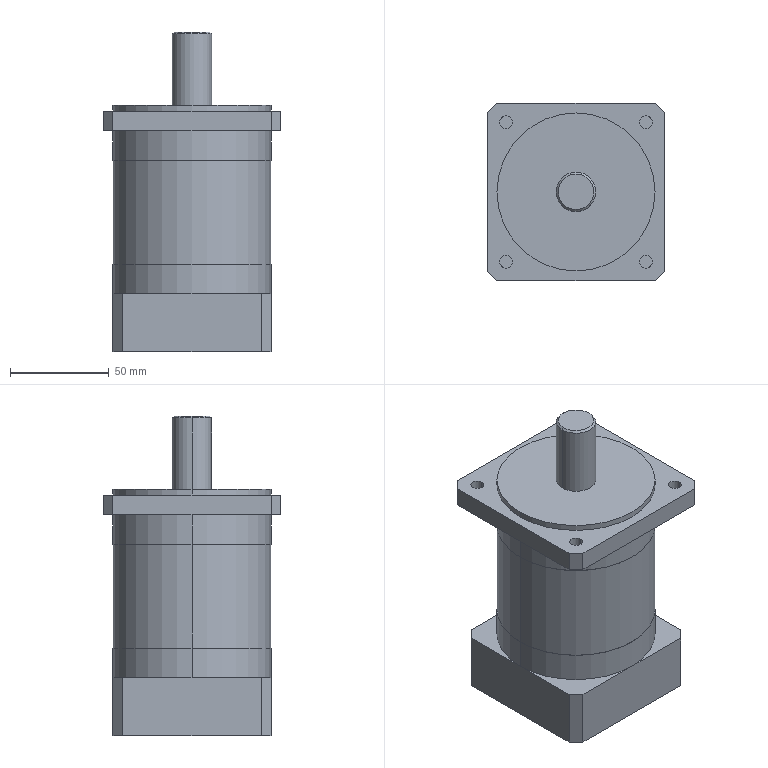Part | STEP file | PL80-40 | 1 solid | 69 faces | box 90 x 90 x 162 mm | volume 688452 mm3 | cylinder 30 | plane 29 | cone 10 | commonest cylinder face diameters 5 x8 6.5 x8 80 x6 16 x2 20 x2 70 x2